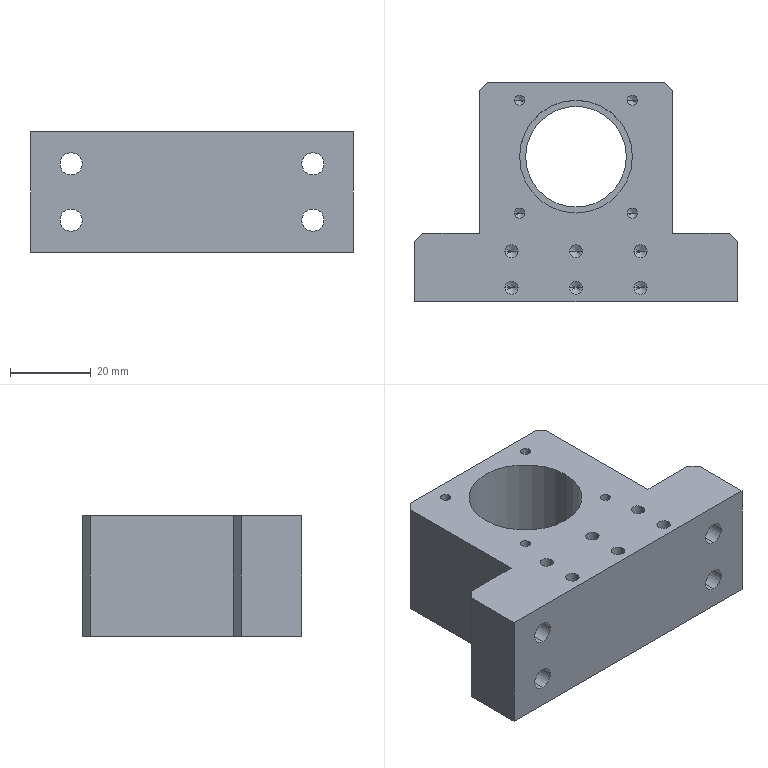Part | STEP file | lead screw fixing block - COMPANY_A version | 1 solid | 83 faces | box 80 x 54.5 x 30 mm | volume 73786 mm3 | cylinder 40 | cone 28 | plane 15 | commonest cylinder face diameters 3.3 x16 2.5 x12 5.5 x8 25 x2 28 x2